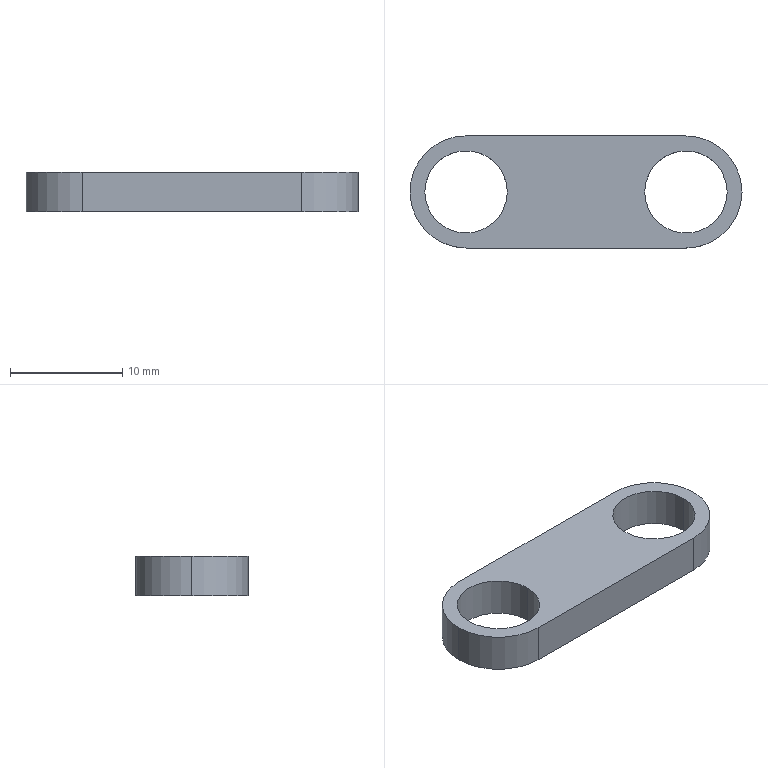Part | SolidWorks | features Cut 1, Extrusion 1 | 1 solid | 11 faces | box 29.602 x 10.008 x 3.5 mm | volume 664.007 mm3 | cylinder 7 | plane 4 | commonest cylinder face diameters 7.349 x4 10 x3
STEP:
#1=CARTESIAN_POINT('',(30.74,0.,3.5));
#2=VERTEX_POINT('',#1);
#3=CARTESIAN_POINT('',(23.391,0.,3.5));
#4=VERTEX_POINT('',#3);
#5=CARTESIAN_POINT('',(27.066,0.,3.5));
#6=DIRECTION('',(0.,0.,-1.));
#7=DIRECTION('',(1.,0.,0.));
#8=AXIS2_PLACEMENT_3D('',#5,#6,#7);
#9=CIRCLE('',#8,3.675);
#10=EDGE_CURVE('',#2,#4,#9,.T.);
#11=ORIENTED_EDGE('',*,*,#10,.F.);
#12=CARTESIAN_POINT('',(30.74,0.,0.));
#13=VERTEX_POINT('',#12);
#14=CARTESIAN_POINT('',(30.74,0.,13.893));
#15=DIRECTION('',(0.,0.,-1.));
#16=VECTOR('',#15,1000.);
#17=LINE('',#14,#16);
#18=EDGE_CURVE('',#2,#13,#17,.T.);
#19=ORIENTED_EDGE('',*,*,#18,.T.);
#20=CARTESIAN_POINT('',(23.391,0.,0.));
#21=VERTEX_POINT('',#20);
#22=CARTESIAN_POINT('',(27.066,0.,0.));
#23=DIRECTION('',(0.,0.,-1.));
#24=DIRECTION('',(-1.,0.,0.));
#25=AXIS2_PLACEMENT_3D('',#22,#23,#24);
#26=CIRCLE('',#25,3.675);
#27=EDGE_CURVE('',#13,#21,#26,.T.);
#28=ORIENTED_EDGE('',*,*,#27,.T.);
#29=CARTESIAN_POINT('',(23.391,0.,13.893));
#30=DIRECTION('',(0.,0.,-1.));
#31=VECTOR('',#30,1000.);
#32=LINE('',#29,#31);
#33=EDGE_CURVE('',#4,#21,#32,.T.);
#34=ORIENTED_EDGE('',*,*,#33,.F.);
#35=EDGE_LOOP('',(#11,#19,#28,#34));
#36=FACE_OUTER_BOUND('',#35,.T.);
#37=CARTESIAN_POINT('',(27.066,0.,13.893));
#38=DIRECTION('',(0.,0.,-1.));
#39=DIRECTION('',(-1.,0.,0.));
#40=AXIS2_PLACEMENT_3D('',#37,#38,#39);
#41=CYLINDRICAL_SURFACE('',#40,3.675);
#42=ADVANCED_FACE('',(#36),#41,.F.);
#43=CARTESIAN_POINT('',(11.139,0.007713,3.5));
#44=VERTEX_POINT('',#43);
#45=CARTESIAN_POINT('',(3.789,0.007713,3.5));
#46=VERTEX_POINT('',#45);
#47=CARTESIAN_POINT('',(7.464,0.007713,3.5));
#48=DIRECTION('',(0.,0.,-1.));
#49=DIRECTION('',(1.,0.,0.));
#50=AXIS2_PLACEMENT_3D('',#47,#48,#49);
#51=CIRCLE('',#50,3.675);
#52=EDGE_CURVE('',#44,#46,#51,.T.);
#53=ORIENTED_EDGE('',*,*,#52,.F.);
#54=CARTESIAN_POINT('',(11.139,0.007713,0.));
#55=VERTEX_POINT('',#54);
#56=CARTESIAN_POINT('',(11.139,0.007713,13.893));
#57=DIRECTION('',(0.,0.,-1.));
#58=VECTOR('',#57,1000.);
#59=LINE('',#56,#58);
#60=EDGE_CURVE('',#44,#55,#59,.T.);
#61=ORIENTED_EDGE('',*,*,#60,.T.);
#62=CARTESIAN_POINT('',(3.789,0.007713,0.));
#63=VERTEX_POINT('',#62);
#64=CARTESIAN_POINT('',(7.464,0.007713,0.));
#65=DIRECTION('',(0.,0.,-1.));
#66=DIRECTION('',(-1.,0.,0.));
#67=AXIS2_PLACEMENT_3D('',#64,#65,#66);
#68=CIRCLE('',#67,3.675);
#69=EDGE_CURVE('',#55,#63,#68,.T.);
#70=ORIENTED_EDGE('',*,*,#69,.T.);
#71=CARTESIAN_POINT('',(3.789,0.007713,13.893));
#72=DIRECTION('',(0.,0.,-1.));
#73=VECTOR('',#72,1000.);
#74=LINE('',#71,#73);
#75=EDGE_CURVE('',#46,#63,#74,.T.);
#76=ORIENTED_EDGE('',*,*,#75,.F.);
#77=EDGE_LOOP('',(#53,#61,#70,#76));
#78=FACE_OUTER_BOUND('',#77,.T.);
#79=CARTESIAN_POINT('',(7.464,0.007713,13.893));
#80=DIRECTION('',(0.,0.,-1.));
#81=DIRECTION('',(-1.,0.,0.));
#82=AXIS2_PLACEMENT_3D('',#79,#80,#81);
#83=CYLINDRICAL_SURFACE('',#82,3.675);
#84=ADVANCED_FACE('',(#78),#83,.F.);
#85=CARTESIAN_POINT('',(2.464,0.007713,3.5));
#86=VERTEX_POINT('',#85);
#87=CARTESIAN_POINT('',(7.462,-4.992,3.5));
#88=VERTEX_POINT('',#87);
#89=CARTESIAN_POINT('',(7.464,0.007713,3.5));
#90=DIRECTION('',(0.,0.,1.));
#91=DIRECTION('',(1.,0.,0.));
#92=AXIS2_PLACEMENT_3D('',#89,#90,#91);
#93=CIRCLE('',#92,5.);
#94=EDGE_CURVE('',#86,#88,#93,.T.);
#95=ORIENTED_EDGE('',*,*,#94,.F.);
#96=CARTESIAN_POINT('',(2.464,0.007713,0.));
#97=VERTEX_POINT('',#96);
#98=CARTESIAN_POINT('',(2.464,0.007713,34.748));
#99=DIRECTION('',(0.,0.,-1.));
#100=VECTOR('',#99,1000.);
#101=LINE('',#98,#100);
#102=EDGE_CURVE('',#86,#97,#101,.T.);
#103=ORIENTED_EDGE('',*,*,#102,.T.);
#104=CARTESIAN_POINT('',(7.462,-4.992,0.));
#105=VERTEX_POINT('',#104);
#106=CARTESIAN_POINT('',(7.464,0.007713,0.));
#107=DIRECTION('',(0.,0.,1.));
#108=DIRECTION('',(1.,0.,0.));
#109=AXIS2_PLACEMENT_3D('',#106,#107,#108);
#110=CIRCLE('',#109,5.);
#111=EDGE_CURVE('',#97,#105,#110,.T.);
#112=ORIENTED_EDGE('',*,*,#111,.T.);
#113=CARTESIAN_POINT('',(7.462,-4.992,34.748));
#114=DIRECTION('',(0.,0.,-1.));
#115=VECTOR('',#114,1000.);
#116=LINE('',#113,#115);
#117=EDGE_CURVE('',#88,#105,#116,.T.);
#118=ORIENTED_EDGE('',*,*,#117,.F.);
#119=EDGE_LOOP('',(#95,#103,#112,#118));
#120=FACE_OUTER_BOUND('',#119,.T.);
#121=CARTESIAN_POINT('',(7.464,0.007713,34.748));
#122=DIRECTION('',(0.,0.,-1.));
#123=DIRECTION('',(-1.,0.,0.));
#124=AXIS2_PLACEMENT_3D('',#121,#122,#123);
#125=CYLINDRICAL_SURFACE('',#124,5.);
#126=ADVANCED_FACE('',(#120),#125,.T.);
#127=CARTESIAN_POINT('',(27.064,-5.,3.5));
#128=VERTEX_POINT('',#127);
#129=CARTESIAN_POINT('',(7.462,-4.992,3.5));
#130=DIRECTION('',(1.,-0.0003935,0.));
#131=VECTOR('',#130,1000.);
#132=LINE('',#129,#131);
#133=EDGE_CURVE('',#88,#128,#132,.T.);
#134=ORIENTED_EDGE('',*,*,#133,.F.);
#135=ORIENTED_EDGE('',*,*,#117,.T.);
#136=CARTESIAN_POINT('',(27.064,-5.,0.));
#137=VERTEX_POINT('',#136);
#138=CARTESIAN_POINT('',(7.462,-4.992,0.));
#139=DIRECTION('',(1.,-0.0003935,0.));
#140=VECTOR('',#139,1000.);
#141=LINE('',#138,#140);
#142=EDGE_CURVE('',#105,#137,#141,.T.);
#143=ORIENTED_EDGE('',*,*,#142,.T.);
#144=CARTESIAN_POINT('',(27.064,-5.,34.748));
#145=DIRECTION('',(0.,0.,-1.));
#146=VECTOR('',#145,1000.);
#147=LINE('',#144,#146);
#148=EDGE_CURVE('',#128,#137,#147,.T.);
#149=ORIENTED_EDGE('',*,*,#148,.F.);
#150=EDGE_LOOP('',(#134,#135,#143,#149));
#151=FACE_OUTER_BOUND('',#150,.T.);
#152=CARTESIAN_POINT('',(7.462,-4.992,34.748));
#153=DIRECTION('',(0.0003935,1.,0.));
#154=DIRECTION('',(-1.,0.0003935,0.));
#155=AXIS2_PLACEMENT_3D('',#152,#153,#154);
#156=PLANE('',#155);
#157=ADVANCED_FACE('',(#151),#156,.F.);
#158=CARTESIAN_POINT('',(27.068,5.,3.5));
#159=VERTEX_POINT('',#158);
#160=CARTESIAN_POINT('',(27.066,0.,3.5));
#161=DIRECTION('',(0.,0.,1.));
#162=DIRECTION('',(1.,0.,0.));
#163=AXIS2_PLACEMENT_3D('',#160,#161,#162);
#164=CIRCLE('',#163,5.);
#165=EDGE_CURVE('',#128,#159,#164,.T.);
#166=ORIENTED_EDGE('',*,*,#165,.F.);
#167=ORIENTED_EDGE('',*,*,#148,.T.);
#168=CARTESIAN_POINT('',(27.068,5.,0.));
#169=VERTEX_POINT('',#168);
#170=CARTESIAN_POINT('',(27.066,0.,0.));
#171=DIRECTION('',(0.,0.,1.));
#172=DIRECTION('',(1.,0.,0.));
#173=AXIS2_PLACEMENT_3D('',#170,#171,#172);
#174=CIRCLE('',#173,5.);
#175=EDGE_CURVE('',#137,#169,#174,.T.);
#176=ORIENTED_EDGE('',*,*,#175,.T.);
#177=CARTESIAN_POINT('',(27.068,5.,34.748));
#178=DIRECTION('',(0.,0.,-1.));
#179=VECTOR('',#178,1000.);
#180=LINE('',#177,#179);
#181=EDGE_CURVE('',#159,#169,#180,.T.);
#182=ORIENTED_EDGE('',*,*,#181,.F.);
#183=EDGE_LOOP('',(#166,#167,#176,#182));
#184=FACE_OUTER_BOUND('',#183,.T.);
#185=CARTESIAN_POINT('',(27.066,0.,34.748));
#186=DIRECTION('',(0.,0.,-1.));
#187=DIRECTION('',(-1.,0.,0.));
#188=AXIS2_PLACEMENT_3D('',#185,#186,#187);
#189=CYLINDRICAL_SURFACE('',#188,5.);
#190=ADVANCED_FACE('',(#184),#189,.T.);
#191=CARTESIAN_POINT('',(7.466,5.008,3.5));
#192=VERTEX_POINT('',#191);
#193=CARTESIAN_POINT('',(7.466,5.008,0.));
#194=VERTEX_POINT('',#193);
#195=CARTESIAN_POINT('',(7.466,5.008,34.748));
#196=DIRECTION('',(0.,0.,-1.));
#197=VECTOR('',#196,1000.);
#198=LINE('',#195,#197);
#199=EDGE_CURVE('',#192,#194,#198,.T.);
#200=ORIENTED_EDGE('',*,*,#199,.F.);
#201=CARTESIAN_POINT('',(7.466,5.008,3.5));
#202=DIRECTION('',(1.,-0.0003935,0.));
#203=VECTOR('',#202,1000.);
#204=LINE('',#201,#203);
#205=EDGE_CURVE('',#192,#159,#204,.T.);
#206=ORIENTED_EDGE('',*,*,#205,.T.);
#207=ORIENTED_EDGE('',*,*,#181,.T.);
#208=CARTESIAN_POINT('',(7.466,5.008,0.));
#209=DIRECTION('',(1.,-0.0003935,0.));
#210=VECTOR('',#209,1000.);
#211=LINE('',#208,#210);
#212=EDGE_CURVE('',#194,#169,#211,.T.);
#213=ORIENTED_EDGE('',*,*,#212,.F.);
#214=EDGE_LOOP('',(#200,#206,#207,#213));
#215=FACE_OUTER_BOUND('',#214,.T.);
#216=CARTESIAN_POINT('',(7.466,5.008,34.748));
#217=DIRECTION('',(0.0003935,1.,0.));
#218=DIRECTION('',(-1.,0.0003935,0.));
#219=AXIS2_PLACEMENT_3D('',#216,#217,#218);
#220=PLANE('',#219);
#221=ADVANCED_FACE('',(#215),#220,.T.);
#222=ORIENTED_EDGE('',*,*,#102,.F.);
#223=CARTESIAN_POINT('',(7.464,0.007713,3.5));
#224=DIRECTION('',(0.,0.,1.));
#225=DIRECTION('',(1.,0.,0.));
#226=AXIS2_PLACEMENT_3D('',#223,#224,#225);
#227=CIRCLE('',#226,5.);
#228=EDGE_CURVE('',#192,#86,#227,.T.);
#229=ORIENTED_EDGE('',*,*,#228,.F.);
#230=ORIENTED_EDGE('',*,*,#199,.T.);
#231=CARTESIAN_POINT('',(7.464,0.007713,0.));
#232=DIRECTION('',(0.,0.,1.));
#233=DIRECTION('',(1.,0.,0.));
#234=AXIS2_PLACEMENT_3D('',#231,#232,#233);
#235=CIRCLE('',#234,5.);
#236=EDGE_CURVE('',#194,#97,#235,.T.);
#237=ORIENTED_EDGE('',*,*,#236,.T.);
#238=EDGE_LOOP('',(#222,#229,#230,#237));
#239=FACE_OUTER_BOUND('',#238,.T.);
#240=CARTESIAN_POINT('',(7.464,0.007713,34.748));
#241=DIRECTION('',(0.,0.,-1.));
#242=DIRECTION('',(-1.,0.,0.));
#243=AXIS2_PLACEMENT_3D('',#240,#241,#242);
#244=CYLINDRICAL_SURFACE('',#243,5.);
#245=ADVANCED_FACE('',(#239),#244,.T.);
#246=CARTESIAN_POINT('',(27.066,0.,0.));
#247=DIRECTION('',(0.,0.,-1.));
#248=DIRECTION('',(-1.,0.,0.));
#249=AXIS2_PLACEMENT_3D('',#246,#247,#248);
#250=CIRCLE('',#249,3.675);
#251=EDGE_CURVE('',#21,#13,#250,.T.);
#252=ORIENTED_EDGE('',*,*,#251,.F.);
#253=ORIENTED_EDGE('',*,*,#27,.F.);
#254=EDGE_LOOP('',(#252,#253));
#255=FACE_BOUND('',#254,.T.);
#256=CARTESIAN_POINT('',(7.464,0.007713,0.));
#257=DIRECTION('',(0.,0.,-1.));
#258=DIRECTION('',(-1.,0.,0.));
#259=AXIS2_PLACEMENT_3D('',#256,#257,#258);
#260=CIRCLE('',#259,3.675);
#261=EDGE_CURVE('',#63,#55,#260,.T.);
#262=ORIENTED_EDGE('',*,*,#261,.F.);
#263=ORIENTED_EDGE('',*,*,#69,.F.);
#264=EDGE_LOOP('',(#262,#263));
#265=FACE_BOUND('',#264,.T.);
#266=ORIENTED_EDGE('',*,*,#142,.F.);
#267=ORIENTED_EDGE('',*,*,#111,.F.);
#268=ORIENTED_EDGE('',*,*,#236,.F.);
#269=ORIENTED_EDGE('',*,*,#212,.T.);
#270=ORIENTED_EDGE('',*,*,#175,.F.);
#271=EDGE_LOOP('',(#266,#267,#268,#269,#270));
#272=FACE_OUTER_BOUND('',#271,.T.);
#273=CARTESIAN_POINT('',(27.066,0.,0.));
#274=DIRECTION('',(0.,0.,1.));
#275=DIRECTION('',(1.,0.,0.));
#276=AXIS2_PLACEMENT_3D('',#273,#274,#275);
#277=PLANE('',#276);
#278=ADVANCED_FACE('',(#255,#265,#272),#277,.F.);
#279=CARTESIAN_POINT('',(27.066,0.,3.5));
#280=DIRECTION('',(0.,0.,-1.));
#281=DIRECTION('',(1.,0.,0.));
#282=AXIS2_PLACEMENT_3D('',#279,#280,#281);
#283=CIRCLE('',#282,3.675);
#284=EDGE_CURVE('',#4,#2,#283,.T.);
#285=ORIENTED_EDGE('',*,*,#284,.T.);
#286=ORIENTED_EDGE('',*,*,#10,.T.);
#287=EDGE_LOOP('',(#285,#286));
#288=FACE_BOUND('',#287,.T.);
#289=CARTESIAN_POINT('',(7.464,0.007713,3.5));
#290=DIRECTION('',(0.,0.,-1.));
#291=DIRECTION('',(1.,0.,0.));
#292=AXIS2_PLACEMENT_3D('',#289,#290,#291);
#293=CIRCLE('',#292,3.675);
#294=EDGE_CURVE('',#46,#44,#293,.T.);
#295=ORIENTED_EDGE('',*,*,#294,.T.);
#296=ORIENTED_EDGE('',*,*,#52,.T.);
#297=EDGE_LOOP('',(#295,#296));
#298=FACE_BOUND('',#297,.T.);
#299=ORIENTED_EDGE('',*,*,#228,.T.);
#300=ORIENTED_EDGE('',*,*,#94,.T.);
#301=ORIENTED_EDGE('',*,*,#133,.T.);
#302=ORIENTED_EDGE('',*,*,#165,.T.);
#303=ORIENTED_EDGE('',*,*,#205,.F.);
#304=EDGE_LOOP('',(#299,#300,#301,#302,#303));
#305=FACE_OUTER_BOUND('',#304,.T.);
#306=CARTESIAN_POINT('',(0.,0.,3.5));
#307=DIRECTION('',(0.,0.,1.));
#308=DIRECTION('',(1.,0.,0.));
#309=AXIS2_PLACEMENT_3D('',#306,#307,#308);
#310=PLANE('',#309);
#311=ADVANCED_FACE('',(#288,#298,#305),#310,.T.);
#312=ORIENTED_EDGE('',*,*,#60,.F.);
#313=ORIENTED_EDGE('',*,*,#294,.F.);
#314=ORIENTED_EDGE('',*,*,#75,.T.);
#315=ORIENTED_EDGE('',*,*,#261,.T.);
#316=EDGE_LOOP('',(#312,#313,#314,#315));
#317=FACE_OUTER_BOUND('',#316,.T.);
#318=CARTESIAN_POINT('',(7.464,0.007713,13.893));
#319=DIRECTION('',(0.,0.,-1.));
#320=DIRECTION('',(-1.,0.,0.));
#321=AXIS2_PLACEMENT_3D('',#318,#319,#320);
#322=CYLINDRICAL_SURFACE('',#321,3.675);
#323=ADVANCED_FACE('',(#317),#322,.F.);
#324=ORIENTED_EDGE('',*,*,#18,.F.);
#325=ORIENTED_EDGE('',*,*,#284,.F.);
#326=ORIENTED_EDGE('',*,*,#33,.T.);
#327=ORIENTED_EDGE('',*,*,#251,.T.);
#328=EDGE_LOOP('',(#324,#325,#326,#327));
#329=FACE_OUTER_BOUND('',#328,.T.);
#330=CARTESIAN_POINT('',(27.066,0.,13.893));
#331=DIRECTION('',(0.,0.,-1.));
#332=DIRECTION('',(-1.,0.,0.));
#333=AXIS2_PLACEMENT_3D('',#330,#331,#332);
#334=CYLINDRICAL_SURFACE('',#333,3.675);
#335=ADVANCED_FACE('',(#329),#334,.F.);
#336=CLOSED_SHELL('',(#42,#84,#126,#157,#190,#221,#245,#278,#311,#323,#335));
#337=MANIFOLD_SOLID_BREP('',#336);
#338=CARTESIAN_POINT('',(0.,0.,0.));
#339=DIRECTION('',(0.,0.,1.));
#340=DIRECTION('',(1.,0.,0.));
#341=AXIS2_PLACEMENT_3D('',#338,#339,#340);
#342=(LENGTH_UNIT()NAMED_UNIT(*)SI_UNIT(.MILLI.,.METRE.));
#343=UNCERTAINTY_MEASURE_WITH_UNIT(LENGTH_MEASURE(0.00001),#342,'','');
#344=(NAMED_UNIT(*)PLANE_ANGLE_UNIT()SI_UNIT($,.RADIAN.));
#345=(NAMED_UNIT(*)SI_UNIT($,.STERADIAN.)SOLID_ANGLE_UNIT());
#346=(GEOMETRIC_REPRESENTATION_CONTEXT(3)GLOBAL_UNCERTAINTY_ASSIGNED_CONTEXT((#343))GLOBAL_UNIT_ASSIGNED_CONTEXT((#342,#344,#345))REPRESENTATION_CONTEXT('',''));
#347=ADVANCED_BREP_SHAPE_REPRESENTATION('',(#337,#341),#346);